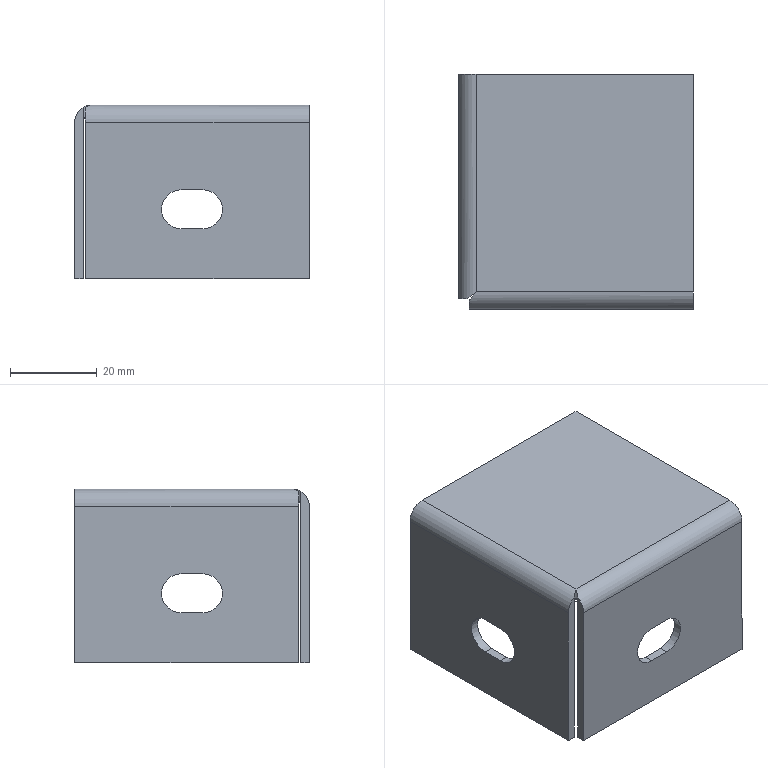Part | STEP file | 750038245 | 1 solid | 26 faces | box 54 x 54 x 40 mm | volume 12946 mm3 | plane 18 | cylinder 8 | commonest cylinder face diameters 9 x4 4 x2 8 x2
STEP:
#1=CARTESIAN_POINT('',(50.,50.,2.));
#2=VERTEX_POINT('',#1);
#3=CARTESIAN_POINT('',(50.,0.,2.));
#4=VERTEX_POINT('',#3);
#5=CARTESIAN_POINT('',(50.,0.,2.));
#6=DIRECTION('',(0.,-1.,0.));
#7=VECTOR('',#6,1000.);
#8=LINE('',#5,#7);
#9=EDGE_CURVE('',#2,#4,#8,.T.);
#10=ORIENTED_EDGE('',*,*,#9,.F.);
#11=CARTESIAN_POINT('',(0.,50.,2.));
#12=VERTEX_POINT('',#11);
#13=CARTESIAN_POINT('',(0.,50.,2.));
#14=DIRECTION('',(1.,0.,0.));
#15=VECTOR('',#14,1000.);
#16=LINE('',#13,#15);
#17=EDGE_CURVE('',#12,#2,#16,.T.);
#18=ORIENTED_EDGE('',*,*,#17,.F.);
#19=CARTESIAN_POINT('',(0.,0.,2.));
#20=VERTEX_POINT('',#19);
#21=CARTESIAN_POINT('',(0.,0.,2.));
#22=DIRECTION('',(0.,1.,0.));
#23=VECTOR('',#22,1000.);
#24=LINE('',#21,#23);
#25=EDGE_CURVE('',#20,#12,#24,.T.);
#26=ORIENTED_EDGE('',*,*,#25,.F.);
#27=CARTESIAN_POINT('',(0.,0.,2.));
#28=DIRECTION('',(-1.,0.,0.));
#29=VECTOR('',#28,1000.);
#30=LINE('',#27,#29);
#31=EDGE_CURVE('',#4,#20,#30,.T.);
#32=ORIENTED_EDGE('',*,*,#31,.F.);
#33=EDGE_LOOP('',(#10,#18,#26,#32));
#34=FACE_OUTER_BOUND('',#33,.T.);
#35=CARTESIAN_POINT('',(0.,0.,2.));
#36=DIRECTION('',(0.,0.,-1.));
#37=DIRECTION('',(-1.,0.,0.));
#38=AXIS2_PLACEMENT_3D('',#35,#36,#37);
#39=PLANE('',#38);
#40=ADVANCED_FACE('',(#34),#39,.F.);
#41=CARTESIAN_POINT('',(-1.5,-4.,-2.));
#42=VERTEX_POINT('',#41);
#43=CARTESIAN_POINT('',(50.,-4.,-2.));
#44=VERTEX_POINT('',#43);
#45=CARTESIAN_POINT('',(50.,-4.,-2.));
#46=DIRECTION('',(1.,0.,0.));
#47=VECTOR('',#46,1000.);
#48=LINE('',#45,#47);
#49=EDGE_CURVE('',#42,#44,#48,.T.);
#50=ORIENTED_EDGE('',*,*,#49,.T.);
#51=CARTESIAN_POINT('',(50.,0.,-2.));
#52=DIRECTION('',(-1.,0.,0.));
#53=DIRECTION('',(0.,0.,1.));
#54=AXIS2_PLACEMENT_3D('',#51,#52,#53);
#55=CIRCLE('',#54,4.);
#56=EDGE_CURVE('',#44,#4,#55,.T.);
#57=ORIENTED_EDGE('',*,*,#56,.T.);
#58=ORIENTED_EDGE('',*,*,#31,.T.);
#59=CARTESIAN_POINT('',(-1.5,-2.,1.464));
#60=VERTEX_POINT('',#59);
#61=CARTESIAN_POINT('',(0.,0.,2.));
#62=CARTESIAN_POINT('',(-0.5297,-0.7062,2.));
#63=CARTESIAN_POINT('',(-1.041,-1.388,1.817));
#64=CARTESIAN_POINT('',(-1.5,-2.,1.464));
#65=(BOUNDED_CURVE()B_SPLINE_CURVE(3,(#61,#62,#63,#64),.UNSPECIFIED.,.F.,.T.)B_SPLINE_CURVE_WITH_KNOTS((4,4),(4.712,5.236),.UNSPECIFIED.)CURVE()GEOMETRIC_REPRESENTATION_ITEM()RATIONAL_B_SPLINE_CURVE((1.,0.9773,0.9773,1.))REPRESENTATION_ITEM(''));
#66=EDGE_CURVE('',#20,#60,#65,.T.);
#67=ORIENTED_EDGE('',*,*,#66,.T.);
#68=CARTESIAN_POINT('',(-1.5,0.,-2.));
#69=DIRECTION('',(1.,0.,0.));
#70=DIRECTION('',(0.,0.,1.));
#71=AXIS2_PLACEMENT_3D('',#68,#69,#70);
#72=CIRCLE('',#71,4.);
#73=EDGE_CURVE('',#60,#42,#72,.T.);
#74=ORIENTED_EDGE('',*,*,#73,.T.);
#75=EDGE_LOOP('',(#50,#57,#58,#67,#74));
#76=FACE_OUTER_BOUND('',#75,.T.);
#77=CARTESIAN_POINT('',(50.,0.,-2.));
#78=DIRECTION('',(-1.,0.,0.));
#79=DIRECTION('',(0.,0.,1.));
#80=AXIS2_PLACEMENT_3D('',#77,#78,#79);
#81=CYLINDRICAL_SURFACE('',#80,4.);
#82=ADVANCED_FACE('',(#76),#81,.T.);
#83=CARTESIAN_POINT('',(50.,0.,0.));
#84=VERTEX_POINT('',#83);
#85=CARTESIAN_POINT('',(50.,50.,0.));
#86=VERTEX_POINT('',#85);
#87=CARTESIAN_POINT('',(50.,50.,0.));
#88=DIRECTION('',(0.,1.,0.));
#89=VECTOR('',#88,1000.);
#90=LINE('',#87,#89);
#91=EDGE_CURVE('',#84,#86,#90,.T.);
#92=ORIENTED_EDGE('',*,*,#91,.T.);
#93=CARTESIAN_POINT('',(50.,50.,2.));
#94=DIRECTION('',(0.,0.,1.));
#95=VECTOR('',#94,1000.);
#96=LINE('',#93,#95);
#97=EDGE_CURVE('',#86,#2,#96,.T.);
#98=ORIENTED_EDGE('',*,*,#97,.T.);
#99=ORIENTED_EDGE('',*,*,#9,.T.);
#100=ORIENTED_EDGE('',*,*,#56,.F.);
#101=CARTESIAN_POINT('',(50.,-4.,-38.));
#102=VERTEX_POINT('',#101);
#103=CARTESIAN_POINT('',(50.,-4.,2.));
#104=DIRECTION('',(0.,0.,-1.));
#105=VECTOR('',#104,1000.);
#106=LINE('',#103,#105);
#107=EDGE_CURVE('',#44,#102,#106,.T.);
#108=ORIENTED_EDGE('',*,*,#107,.T.);
#109=CARTESIAN_POINT('',(50.,-2.,-38.));
#110=VERTEX_POINT('',#109);
#111=CARTESIAN_POINT('',(50.,50.,-38.));
#112=DIRECTION('',(0.,1.,0.));
#113=VECTOR('',#112,1000.);
#114=LINE('',#111,#113);
#115=EDGE_CURVE('',#102,#110,#114,.T.);
#116=ORIENTED_EDGE('',*,*,#115,.T.);
#117=CARTESIAN_POINT('',(50.,-2.,-2.));
#118=VERTEX_POINT('',#117);
#119=CARTESIAN_POINT('',(50.,-2.,2.));
#120=DIRECTION('',(0.,0.,1.));
#121=VECTOR('',#120,1000.);
#122=LINE('',#119,#121);
#123=EDGE_CURVE('',#110,#118,#122,.T.);
#124=ORIENTED_EDGE('',*,*,#123,.T.);
#125=CARTESIAN_POINT('',(50.,0.,-2.));
#126=DIRECTION('',(-1.,0.,0.));
#127=DIRECTION('',(0.,0.,1.));
#128=AXIS2_PLACEMENT_3D('',#125,#126,#127);
#129=CIRCLE('',#128,2.);
#130=EDGE_CURVE('',#118,#84,#129,.T.);
#131=ORIENTED_EDGE('',*,*,#130,.T.);
#132=EDGE_LOOP('',(#92,#98,#99,#100,#108,#116,#124,#131));
#133=FACE_OUTER_BOUND('',#132,.T.);
#134=CARTESIAN_POINT('',(50.,50.,2.));
#135=DIRECTION('',(1.,0.,0.));
#136=DIRECTION('',(0.,1.,0.));
#137=AXIS2_PLACEMENT_3D('',#134,#135,#136);
#138=PLANE('',#137);
#139=ADVANCED_FACE('',(#133),#138,.T.);
#140=ORIENTED_EDGE('',*,*,#97,.F.);
#141=CARTESIAN_POINT('',(0.,50.,0.));
#142=VERTEX_POINT('',#141);
#143=CARTESIAN_POINT('',(0.,50.,0.));
#144=DIRECTION('',(-1.,0.,0.));
#145=VECTOR('',#144,1000.);
#146=LINE('',#143,#145);
#147=EDGE_CURVE('',#86,#142,#146,.T.);
#148=ORIENTED_EDGE('',*,*,#147,.T.);
#149=CARTESIAN_POINT('',(-2.,50.,-2.));
#150=VERTEX_POINT('',#149);
#151=CARTESIAN_POINT('',(0.,50.,-2.));
#152=DIRECTION('',(0.,-1.,0.));
#153=DIRECTION('',(-1.,0.,0.));
#154=AXIS2_PLACEMENT_3D('',#151,#152,#153);
#155=CIRCLE('',#154,2.);
#156=EDGE_CURVE('',#142,#150,#155,.T.);
#157=ORIENTED_EDGE('',*,*,#156,.T.);
#158=CARTESIAN_POINT('',(-2.,50.,-38.));
#159=VERTEX_POINT('',#158);
#160=CARTESIAN_POINT('',(-2.,50.,2.));
#161=DIRECTION('',(0.,0.,-1.));
#162=VECTOR('',#161,1000.);
#163=LINE('',#160,#162);
#164=EDGE_CURVE('',#150,#159,#163,.T.);
#165=ORIENTED_EDGE('',*,*,#164,.T.);
#166=CARTESIAN_POINT('',(-4.,50.,-38.));
#167=VERTEX_POINT('',#166);
#168=CARTESIAN_POINT('',(0.,50.,-38.));
#169=DIRECTION('',(-1.,0.,0.));
#170=VECTOR('',#169,1000.);
#171=LINE('',#168,#170);
#172=EDGE_CURVE('',#159,#167,#171,.T.);
#173=ORIENTED_EDGE('',*,*,#172,.T.);
#174=CARTESIAN_POINT('',(-4.,50.,-2.));
#175=VERTEX_POINT('',#174);
#176=CARTESIAN_POINT('',(-4.,50.,2.));
#177=DIRECTION('',(0.,0.,1.));
#178=VECTOR('',#177,1000.);
#179=LINE('',#176,#178);
#180=EDGE_CURVE('',#167,#175,#179,.T.);
#181=ORIENTED_EDGE('',*,*,#180,.T.);
#182=CARTESIAN_POINT('',(0.,50.,-2.));
#183=DIRECTION('',(0.,-1.,0.));
#184=DIRECTION('',(-1.,0.,0.));
#185=AXIS2_PLACEMENT_3D('',#182,#183,#184);
#186=CIRCLE('',#185,4.);
#187=EDGE_CURVE('',#12,#175,#186,.T.);
#188=ORIENTED_EDGE('',*,*,#187,.F.);
#189=ORIENTED_EDGE('',*,*,#17,.T.);
#190=EDGE_LOOP('',(#140,#148,#157,#165,#173,#181,#188,#189));
#191=FACE_OUTER_BOUND('',#190,.T.);
#192=CARTESIAN_POINT('',(0.,50.,2.));
#193=DIRECTION('',(0.,1.,0.));
#194=DIRECTION('',(0.,0.,1.));
#195=AXIS2_PLACEMENT_3D('',#192,#193,#194);
#196=PLANE('',#195);
#197=ADVANCED_FACE('',(#191),#196,.T.);
#198=CARTESIAN_POINT('',(-4.,-1.5,-2.));
#199=VERTEX_POINT('',#198);
#200=CARTESIAN_POINT('',(-4.,0.,-2.));
#201=DIRECTION('',(0.,-1.,0.));
#202=VECTOR('',#201,1000.);
#203=LINE('',#200,#202);
#204=EDGE_CURVE('',#175,#199,#203,.T.);
#205=ORIENTED_EDGE('',*,*,#204,.T.);
#206=CARTESIAN_POINT('',(-2.,-1.5,1.464));
#207=VERTEX_POINT('',#206);
#208=CARTESIAN_POINT('',(0.,-1.5,-2.));
#209=DIRECTION('',(0.,1.,0.));
#210=DIRECTION('',(-1.,0.,0.));
#211=AXIS2_PLACEMENT_3D('',#208,#209,#210);
#212=CIRCLE('',#211,4.);
#213=EDGE_CURVE('',#199,#207,#212,.T.);
#214=ORIENTED_EDGE('',*,*,#213,.T.);
#215=CARTESIAN_POINT('',(-2.,-1.5,1.464));
#216=CARTESIAN_POINT('',(-1.388,-1.041,1.817));
#217=CARTESIAN_POINT('',(-0.7062,-0.5297,2.));
#218=CARTESIAN_POINT('',(0.,0.,2.));
#219=(BOUNDED_CURVE()B_SPLINE_CURVE(3,(#215,#216,#217,#218),.UNSPECIFIED.,.F.,.F.)B_SPLINE_CURVE_WITH_KNOTS((4,4),(4.189,4.712),.UNSPECIFIED.)CURVE()GEOMETRIC_REPRESENTATION_ITEM()RATIONAL_B_SPLINE_CURVE((1.,0.9773,0.9773,1.))REPRESENTATION_ITEM(''));
#220=EDGE_CURVE('',#207,#20,#219,.T.);
#221=ORIENTED_EDGE('',*,*,#220,.T.);
#222=ORIENTED_EDGE('',*,*,#25,.T.);
#223=ORIENTED_EDGE('',*,*,#187,.T.);
#224=EDGE_LOOP('',(#205,#214,#221,#222,#223));
#225=FACE_OUTER_BOUND('',#224,.T.);
#226=CARTESIAN_POINT('',(0.,0.,-2.));
#227=DIRECTION('',(0.,1.,0.));
#228=DIRECTION('',(-1.,0.,0.));
#229=AXIS2_PLACEMENT_3D('',#226,#227,#228);
#230=CYLINDRICAL_SURFACE('',#229,4.);
#231=ADVANCED_FACE('',(#225),#230,.T.);
#232=CARTESIAN_POINT('',(-1.5,-4.,-38.));
#233=VERTEX_POINT('',#232);
#234=CARTESIAN_POINT('',(50.,-4.,-38.));
#235=DIRECTION('',(-1.,0.,0.));
#236=VECTOR('',#235,1000.);
#237=LINE('',#234,#236);
#238=EDGE_CURVE('',#102,#233,#237,.T.);
#239=ORIENTED_EDGE('',*,*,#238,.F.);
#240=ORIENTED_EDGE('',*,*,#107,.F.);
#241=ORIENTED_EDGE('',*,*,#49,.F.);
#242=CARTESIAN_POINT('',(-1.5,-4.,-2.));
#243=DIRECTION('',(0.,0.,1.));
#244=VECTOR('',#243,1000.);
#245=LINE('',#242,#244);
#246=EDGE_CURVE('',#233,#42,#245,.T.);
#247=ORIENTED_EDGE('',*,*,#246,.F.);
#248=EDGE_LOOP('',(#239,#240,#241,#247));
#249=FACE_OUTER_BOUND('',#248,.T.);
#250=CARTESIAN_POINT('',(25.5,-4.,-17.5));
#251=VERTEX_POINT('',#250);
#252=CARTESIAN_POINT('',(20.5,-4.,-17.5));
#253=VERTEX_POINT('',#252);
#254=CARTESIAN_POINT('',(50.,-4.,-17.5));
#255=DIRECTION('',(-1.,0.,0.));
#256=VECTOR('',#255,1000.);
#257=LINE('',#254,#256);
#258=EDGE_CURVE('',#251,#253,#257,.T.);
#259=ORIENTED_EDGE('',*,*,#258,.F.);
#260=CARTESIAN_POINT('',(25.5,-4.,-26.5));
#261=VERTEX_POINT('',#260);
#262=CARTESIAN_POINT('',(25.5,-4.,-22.));
#263=DIRECTION('',(0.,-1.,0.));
#264=DIRECTION('',(0.,0.,-1.));
#265=AXIS2_PLACEMENT_3D('',#262,#263,#264);
#266=CIRCLE('',#265,4.5);
#267=EDGE_CURVE('',#261,#251,#266,.T.);
#268=ORIENTED_EDGE('',*,*,#267,.F.);
#269=CARTESIAN_POINT('',(20.5,-4.,-26.5));
#270=VERTEX_POINT('',#269);
#271=CARTESIAN_POINT('',(50.,-4.,-26.5));
#272=DIRECTION('',(1.,0.,0.));
#273=VECTOR('',#272,1000.);
#274=LINE('',#271,#273);
#275=EDGE_CURVE('',#270,#261,#274,.T.);
#276=ORIENTED_EDGE('',*,*,#275,.F.);
#277=CARTESIAN_POINT('',(20.5,-4.,-22.));
#278=DIRECTION('',(0.,-1.,0.));
#279=DIRECTION('',(0.,0.,-1.));
#280=AXIS2_PLACEMENT_3D('',#277,#278,#279);
#281=CIRCLE('',#280,4.5);
#282=EDGE_CURVE('',#253,#270,#281,.T.);
#283=ORIENTED_EDGE('',*,*,#282,.F.);
#284=EDGE_LOOP('',(#259,#268,#276,#283));
#285=FACE_BOUND('',#284,.T.);
#286=CARTESIAN_POINT('',(50.,-4.,-2.));
#287=DIRECTION('',(0.,1.,0.));
#288=DIRECTION('',(0.,0.,1.));
#289=AXIS2_PLACEMENT_3D('',#286,#287,#288);
#290=PLANE('',#289);
#291=ADVANCED_FACE('',(#249,#285),#290,.F.);
#292=CARTESIAN_POINT('',(-1.5,-2.,-2.));
#293=VERTEX_POINT('',#292);
#294=CARTESIAN_POINT('',(-1.5,-2.,-38.));
#295=VERTEX_POINT('',#294);
#296=CARTESIAN_POINT('',(-1.5,-2.,2.));
#297=DIRECTION('',(0.,0.,-1.));
#298=VECTOR('',#297,1000.);
#299=LINE('',#296,#298);
#300=EDGE_CURVE('',#293,#295,#299,.T.);
#301=ORIENTED_EDGE('',*,*,#300,.T.);
#302=CARTESIAN_POINT('',(-1.5,0.,-38.));
#303=DIRECTION('',(0.,-1.,0.));
#304=VECTOR('',#303,1000.);
#305=LINE('',#302,#304);
#306=EDGE_CURVE('',#295,#233,#305,.T.);
#307=ORIENTED_EDGE('',*,*,#306,.T.);
#308=ORIENTED_EDGE('',*,*,#246,.T.);
#309=ORIENTED_EDGE('',*,*,#73,.F.);
#310=CARTESIAN_POINT('',(-1.5,-2.,2.));
#311=DIRECTION('',(0.,0.,-1.));
#312=VECTOR('',#311,1000.);
#313=LINE('',#310,#312);
#314=EDGE_CURVE('',#60,#293,#313,.T.);
#315=ORIENTED_EDGE('',*,*,#314,.T.);
#316=EDGE_LOOP('',(#301,#307,#308,#309,#315));
#317=FACE_OUTER_BOUND('',#316,.T.);
#318=CARTESIAN_POINT('',(-1.5,0.,2.));
#319=DIRECTION('',(-1.,0.,0.));
#320=DIRECTION('',(0.,-1.,0.));
#321=AXIS2_PLACEMENT_3D('',#318,#319,#320);
#322=PLANE('',#321);
#323=ADVANCED_FACE('',(#317),#322,.T.);
#324=CARTESIAN_POINT('',(0.,0.,0.));
#325=VERTEX_POINT('',#324);
#326=CARTESIAN_POINT('',(-1.5,-2.,-2.));
#327=CARTESIAN_POINT('',(-1.5,-2.,-0.8284));
#328=CARTESIAN_POINT('',(-0.8787,-1.172,0.));
#329=CARTESIAN_POINT('',(0.,0.,0.));
#330=(BOUNDED_CURVE()B_SPLINE_CURVE(3,(#326,#327,#328,#329),.UNSPECIFIED.,.F.,.F.)B_SPLINE_CURVE_WITH_KNOTS((4,4),(0.,1.571),.UNSPECIFIED.)CURVE()GEOMETRIC_REPRESENTATION_ITEM()RATIONAL_B_SPLINE_CURVE((1.,0.8047,0.8047,1.))REPRESENTATION_ITEM(''));
#331=EDGE_CURVE('',#293,#325,#330,.T.);
#332=ORIENTED_EDGE('',*,*,#331,.F.);
#333=ORIENTED_EDGE('',*,*,#314,.F.);
#334=ORIENTED_EDGE('',*,*,#66,.F.);
#335=CARTESIAN_POINT('',(0.,0.,1002.));
#336=DIRECTION('',(0.,0.,1.));
#337=VECTOR('',#336,1000.);
#338=LINE('',#335,#337);
#339=EDGE_CURVE('',#325,#20,#338,.T.);
#340=ORIENTED_EDGE('',*,*,#339,.F.);
#341=EDGE_LOOP('',(#332,#333,#334,#340));
#342=FACE_OUTER_BOUND('',#341,.T.);
#343=CARTESIAN_POINT('',(600.,800.,1002.));
#344=DIRECTION('',(0.8,-0.6,0.));
#345=DIRECTION('',(0.6,0.8,0.));
#346=AXIS2_PLACEMENT_3D('',#343,#344,#345);
#347=PLANE('',#346);
#348=ADVANCED_FACE('',(#342),#347,.F.);
#349=ORIENTED_EDGE('',*,*,#147,.F.);
#350=ORIENTED_EDGE('',*,*,#91,.F.);
#351=CARTESIAN_POINT('',(0.,0.,0.));
#352=DIRECTION('',(-1.,0.,0.));
#353=VECTOR('',#352,1000.);
#354=LINE('',#351,#353);
#355=EDGE_CURVE('',#84,#325,#354,.T.);
#356=ORIENTED_EDGE('',*,*,#355,.T.);
#357=CARTESIAN_POINT('',(0.,0.,0.));
#358=DIRECTION('',(0.,1.,0.));
#359=VECTOR('',#358,1000.);
#360=LINE('',#357,#359);
#361=EDGE_CURVE('',#325,#142,#360,.T.);
#362=ORIENTED_EDGE('',*,*,#361,.T.);
#363=EDGE_LOOP('',(#349,#350,#356,#362));
#364=FACE_OUTER_BOUND('',#363,.T.);
#365=CARTESIAN_POINT('',(0.,0.,0.));
#366=DIRECTION('',(0.,0.,-1.));
#367=DIRECTION('',(-1.,0.,0.));
#368=AXIS2_PLACEMENT_3D('',#365,#366,#367);
#369=PLANE('',#368);
#370=ADVANCED_FACE('',(#364),#369,.T.);
#371=CARTESIAN_POINT('',(-4.,-1.5,-38.));
#372=VERTEX_POINT('',#371);
#373=CARTESIAN_POINT('',(-4.,-1.5,-2.));
#374=DIRECTION('',(0.,0.,-1.));
#375=VECTOR('',#374,1000.);
#376=LINE('',#373,#375);
#377=EDGE_CURVE('',#199,#372,#376,.T.);
#378=ORIENTED_EDGE('',*,*,#377,.T.);
#379=CARTESIAN_POINT('',(-2.,-1.5,-38.));
#380=VERTEX_POINT('',#379);
#381=CARTESIAN_POINT('',(-2.,-1.5,-38.));
#382=DIRECTION('',(1.,0.,0.));
#383=VECTOR('',#382,1000.);
#384=LINE('',#381,#383);
#385=EDGE_CURVE('',#372,#380,#384,.T.);
#386=ORIENTED_EDGE('',*,*,#385,.T.);
#387=CARTESIAN_POINT('',(-2.,-1.5,-2.));
#388=VERTEX_POINT('',#387);
#389=CARTESIAN_POINT('',(-2.,-1.5,-2.));
#390=DIRECTION('',(0.,0.,1.));
#391=VECTOR('',#390,1000.);
#392=LINE('',#389,#391);
#393=EDGE_CURVE('',#380,#388,#392,.T.);
#394=ORIENTED_EDGE('',*,*,#393,.T.);
#395=CARTESIAN_POINT('',(-2.,-1.5,-2.));
#396=DIRECTION('',(0.,0.,1.));
#397=VECTOR('',#396,1000.);
#398=LINE('',#395,#397);
#399=EDGE_CURVE('',#388,#207,#398,.T.);
#400=ORIENTED_EDGE('',*,*,#399,.T.);
#401=ORIENTED_EDGE('',*,*,#213,.F.);
#402=EDGE_LOOP('',(#378,#386,#394,#400,#401));
#403=FACE_OUTER_BOUND('',#402,.T.);
#404=CARTESIAN_POINT('',(-2.,-1.5,-2.));
#405=DIRECTION('',(0.,-1.,0.));
#406=DIRECTION('',(1.,0.,0.));
#407=AXIS2_PLACEMENT_3D('',#404,#405,#406);
#408=PLANE('',#407);
#409=ADVANCED_FACE('',(#403),#408,.T.);
#410=CARTESIAN_POINT('',(-4.,0.,-38.));
#411=DIRECTION('',(0.,1.,0.));
#412=VECTOR('',#411,1000.);
#413=LINE('',#410,#412);
#414=EDGE_CURVE('',#372,#167,#413,.T.);
#415=ORIENTED_EDGE('',*,*,#414,.F.);
#416=ORIENTED_EDGE('',*,*,#377,.F.);
#417=ORIENTED_EDGE('',*,*,#204,.F.);
#418=ORIENTED_EDGE('',*,*,#180,.F.);
#419=EDGE_LOOP('',(#415,#416,#417,#418));
#420=FACE_OUTER_BOUND('',#419,.T.);
#421=CARTESIAN_POINT('',(-4.,25.5,-26.5));
#422=VERTEX_POINT('',#421);
#423=CARTESIAN_POINT('',(-4.,20.5,-26.5));
#424=VERTEX_POINT('',#423);
#425=CARTESIAN_POINT('',(-4.,0.,-26.5));
#426=DIRECTION('',(0.,-1.,0.));
#427=VECTOR('',#426,1000.);
#428=LINE('',#425,#427);
#429=EDGE_CURVE('',#422,#424,#428,.T.);
#430=ORIENTED_EDGE('',*,*,#429,.F.);
#431=CARTESIAN_POINT('',(-4.,25.5,-17.5));
#432=VERTEX_POINT('',#431);
#433=CARTESIAN_POINT('',(-4.,25.5,-22.));
#434=DIRECTION('',(-1.,0.,0.));
#435=DIRECTION('',(0.,0.,1.));
#436=AXIS2_PLACEMENT_3D('',#433,#434,#435);
#437=CIRCLE('',#436,4.5);
#438=EDGE_CURVE('',#432,#422,#437,.T.);
#439=ORIENTED_EDGE('',*,*,#438,.F.);
#440=CARTESIAN_POINT('',(-4.,20.5,-17.5));
#441=VERTEX_POINT('',#440);
#442=CARTESIAN_POINT('',(-4.,0.,-17.5));
#443=DIRECTION('',(0.,1.,0.));
#444=VECTOR('',#443,1000.);
#445=LINE('',#442,#444);
#446=EDGE_CURVE('',#441,#432,#445,.T.);
#447=ORIENTED_EDGE('',*,*,#446,.F.);
#448=CARTESIAN_POINT('',(-4.,20.5,-22.));
#449=DIRECTION('',(-1.,0.,0.));
#450=DIRECTION('',(0.,0.,1.));
#451=AXIS2_PLACEMENT_3D('',#448,#449,#450);
#452=CIRCLE('',#451,4.5);
#453=EDGE_CURVE('',#424,#441,#452,.T.);
#454=ORIENTED_EDGE('',*,*,#453,.F.);
#455=EDGE_LOOP('',(#430,#439,#447,#454));
#456=FACE_BOUND('',#455,.T.);
#457=CARTESIAN_POINT('',(-4.,0.,-2.));
#458=DIRECTION('',(1.,0.,0.));
#459=DIRECTION('',(0.,0.,-1.));
#460=AXIS2_PLACEMENT_3D('',#457,#458,#459);
#461=PLANE('',#460);
#462=ADVANCED_FACE('',(#420,#456),#461,.F.);
#463=ORIENTED_EDGE('',*,*,#220,.F.);
#464=ORIENTED_EDGE('',*,*,#399,.F.);
#465=CARTESIAN_POINT('',(-2.,-1.5,-2.));
#466=CARTESIAN_POINT('',(-2.,-1.5,-0.8284));
#467=CARTESIAN_POINT('',(-1.172,-0.8787,0.));
#468=CARTESIAN_POINT('',(0.,0.,0.));
#469=(BOUNDED_CURVE()B_SPLINE_CURVE(3,(#465,#466,#467,#468),.UNSPECIFIED.,.F.,.F.)B_SPLINE_CURVE_WITH_KNOTS((4,4),(3.142,4.712),.UNSPECIFIED.)CURVE()GEOMETRIC_REPRESENTATION_ITEM()RATIONAL_B_SPLINE_CURVE((1.,0.8047,0.8047,1.))REPRESENTATION_ITEM(''));
#470=EDGE_CURVE('',#388,#325,#469,.T.);
#471=ORIENTED_EDGE('',*,*,#470,.T.);
#472=ORIENTED_EDGE('',*,*,#339,.T.);
#473=EDGE_LOOP('',(#463,#464,#471,#472));
#474=FACE_OUTER_BOUND('',#473,.T.);
#475=CARTESIAN_POINT('',(800.,600.,1002.));
#476=DIRECTION('',(0.6,-0.8,0.));
#477=DIRECTION('',(0.8,0.6,0.));
#478=AXIS2_PLACEMENT_3D('',#475,#476,#477);
#479=PLANE('',#478);
#480=ADVANCED_FACE('',(#474),#479,.T.);
#481=ORIENTED_EDGE('',*,*,#306,.F.);
#482=CARTESIAN_POINT('',(50.,-2.,-38.));
#483=DIRECTION('',(1.,0.,0.));
#484=VECTOR('',#483,1000.);
#485=LINE('',#482,#484);
#486=EDGE_CURVE('',#295,#110,#485,.T.);
#487=ORIENTED_EDGE('',*,*,#486,.T.);
#488=ORIENTED_EDGE('',*,*,#115,.F.);
#489=ORIENTED_EDGE('',*,*,#238,.T.);
#490=EDGE_LOOP('',(#481,#487,#488,#489));
#491=FACE_OUTER_BOUND('',#490,.T.);
#492=CARTESIAN_POINT('',(50.,-2.,-38.));
#493=DIRECTION('',(0.,0.,-1.));
#494=DIRECTION('',(0.,1.,0.));
#495=AXIS2_PLACEMENT_3D('',#492,#493,#494);
#496=PLANE('',#495);
#497=ADVANCED_FACE('',(#491),#496,.T.);
#498=ORIENTED_EDGE('',*,*,#355,.F.);
#499=ORIENTED_EDGE('',*,*,#130,.F.);
#500=CARTESIAN_POINT('',(50.,-2.,-2.));
#501=DIRECTION('',(1.,0.,0.));
#502=VECTOR('',#501,1000.);
#503=LINE('',#500,#502);
#504=EDGE_CURVE('',#293,#118,#503,.T.);
#505=ORIENTED_EDGE('',*,*,#504,.F.);
#506=ORIENTED_EDGE('',*,*,#331,.T.);
#507=EDGE_LOOP('',(#498,#499,#505,#506));
#508=FACE_OUTER_BOUND('',#507,.T.);
#509=CARTESIAN_POINT('',(50.,0.,-2.));
#510=DIRECTION('',(-1.,0.,0.));
#511=DIRECTION('',(0.,0.,1.));
#512=AXIS2_PLACEMENT_3D('',#509,#510,#511);
#513=CYLINDRICAL_SURFACE('',#512,2.);
#514=ADVANCED_FACE('',(#508),#513,.F.);
#515=ORIENTED_EDGE('',*,*,#123,.F.);
#516=ORIENTED_EDGE('',*,*,#486,.F.);
#517=ORIENTED_EDGE('',*,*,#300,.F.);
#518=ORIENTED_EDGE('',*,*,#504,.T.);
#519=EDGE_LOOP('',(#515,#516,#517,#518));
#520=FACE_OUTER_BOUND('',#519,.T.);
#521=CARTESIAN_POINT('',(20.5,-2.,-26.5));
#522=VERTEX_POINT('',#521);
#523=CARTESIAN_POINT('',(25.5,-2.,-26.5));
#524=VERTEX_POINT('',#523);
#525=CARTESIAN_POINT('',(50.,-2.,-26.5));
#526=DIRECTION('',(1.,0.,0.));
#527=VECTOR('',#526,1000.);
#528=LINE('',#525,#527);
#529=EDGE_CURVE('',#522,#524,#528,.T.);
#530=ORIENTED_EDGE('',*,*,#529,.T.);
#531=CARTESIAN_POINT('',(25.5,-2.,-17.5));
#532=VERTEX_POINT('',#531);
#533=CARTESIAN_POINT('',(25.5,-2.,-22.));
#534=DIRECTION('',(0.,-1.,0.));
#535=DIRECTION('',(0.,0.,-1.));
#536=AXIS2_PLACEMENT_3D('',#533,#534,#535);
#537=CIRCLE('',#536,4.5);
#538=EDGE_CURVE('',#524,#532,#537,.T.);
#539=ORIENTED_EDGE('',*,*,#538,.T.);
#540=CARTESIAN_POINT('',(20.5,-2.,-17.5));
#541=VERTEX_POINT('',#540);
#542=CARTESIAN_POINT('',(50.,-2.,-17.5));
#543=DIRECTION('',(-1.,0.,0.));
#544=VECTOR('',#543,1000.);
#545=LINE('',#542,#544);
#546=EDGE_CURVE('',#532,#541,#545,.T.);
#547=ORIENTED_EDGE('',*,*,#546,.T.);
#548=CARTESIAN_POINT('',(20.5,-2.,-22.));
#549=DIRECTION('',(0.,-1.,0.));
#550=DIRECTION('',(0.,0.,-1.));
#551=AXIS2_PLACEMENT_3D('',#548,#549,#550);
#552=CIRCLE('',#551,4.5);
#553=EDGE_CURVE('',#541,#522,#552,.T.);
#554=ORIENTED_EDGE('',*,*,#553,.T.);
#555=EDGE_LOOP('',(#530,#539,#547,#554));
#556=FACE_BOUND('',#555,.T.);
#557=CARTESIAN_POINT('',(50.,-2.,-2.));
#558=DIRECTION('',(0.,1.,0.));
#559=DIRECTION('',(0.,0.,1.));
#560=AXIS2_PLACEMENT_3D('',#557,#558,#559);
#561=PLANE('',#560);
#562=ADVANCED_FACE('',(#520,#556),#561,.T.);
#563=CARTESIAN_POINT('',(20.5,82.209,-17.5));
#564=DIRECTION('',(0.,1.,0.));
#565=VECTOR('',#564,1000.);
#566=LINE('',#563,#565);
#567=EDGE_CURVE('',#253,#541,#566,.T.);
#568=ORIENTED_EDGE('',*,*,#567,.F.);
#569=ORIENTED_EDGE('',*,*,#282,.T.);
#570=CARTESIAN_POINT('',(20.5,82.209,-26.5));
#571=DIRECTION('',(0.,-1.,0.));
#572=VECTOR('',#571,1000.);
#573=LINE('',#570,#572);
#574=EDGE_CURVE('',#522,#270,#573,.T.);
#575=ORIENTED_EDGE('',*,*,#574,.F.);
#576=ORIENTED_EDGE('',*,*,#553,.F.);
#577=EDGE_LOOP('',(#568,#569,#575,#576));
#578=FACE_OUTER_BOUND('',#577,.T.);
#579=CARTESIAN_POINT('',(20.5,82.209,-22.));
#580=DIRECTION('',(0.,-1.,0.));
#581=DIRECTION('',(0.,0.,-1.));
#582=AXIS2_PLACEMENT_3D('',#579,#580,#581);
#583=CYLINDRICAL_SURFACE('',#582,4.5);
#584=ADVANCED_FACE('',(#578),#583,.F.);
#585=CARTESIAN_POINT('',(25.5,82.209,-17.5));
#586=DIRECTION('',(0.,1.,0.));
#587=VECTOR('',#586,1000.);
#588=LINE('',#585,#587);
#589=EDGE_CURVE('',#251,#532,#588,.T.);
#590=ORIENTED_EDGE('',*,*,#589,.F.);
#591=ORIENTED_EDGE('',*,*,#258,.T.);
#592=ORIENTED_EDGE('',*,*,#567,.T.);
#593=ORIENTED_EDGE('',*,*,#546,.F.);
#594=EDGE_LOOP('',(#590,#591,#592,#593));
#595=FACE_OUTER_BOUND('',#594,.T.);
#596=CARTESIAN_POINT('',(25.5,82.209,-17.5));
#597=DIRECTION('',(0.,0.,1.));
#598=DIRECTION('',(1.,0.,0.));
#599=AXIS2_PLACEMENT_3D('',#596,#597,#598);
#600=PLANE('',#599);
#601=ADVANCED_FACE('',(#595),#600,.F.);
#602=CARTESIAN_POINT('',(25.5,82.209,-26.5));
#603=DIRECTION('',(0.,1.,0.));
#604=VECTOR('',#603,1000.);
#605=LINE('',#602,#604);
#606=EDGE_CURVE('',#261,#524,#605,.T.);
#607=ORIENTED_EDGE('',*,*,#606,.F.);
#608=ORIENTED_EDGE('',*,*,#267,.T.);
#609=ORIENTED_EDGE('',*,*,#589,.T.);
#610=ORIENTED_EDGE('',*,*,#538,.F.);
#611=EDGE_LOOP('',(#607,#608,#609,#610));
#612=FACE_OUTER_BOUND('',#611,.T.);
#613=CARTESIAN_POINT('',(25.5,82.209,-22.));
#614=DIRECTION('',(0.,-1.,0.));
#615=DIRECTION('',(0.,0.,-1.));
#616=AXIS2_PLACEMENT_3D('',#613,#614,#615);
#617=CYLINDRICAL_SURFACE('',#616,4.5);
#618=ADVANCED_FACE('',(#612),#617,.F.);
#619=ORIENTED_EDGE('',*,*,#574,.T.);
#620=ORIENTED_EDGE('',*,*,#275,.T.);
#621=ORIENTED_EDGE('',*,*,#606,.T.);
#622=ORIENTED_EDGE('',*,*,#529,.F.);
#623=EDGE_LOOP('',(#619,#620,#621,#622));
#624=FACE_OUTER_BOUND('',#623,.T.);
#625=CARTESIAN_POINT('',(20.5,82.209,-26.5));
#626=DIRECTION('',(0.,0.,-1.));
#627=DIRECTION('',(-1.,0.,0.));
#628=AXIS2_PLACEMENT_3D('',#625,#626,#627);
#629=PLANE('',#628);
#630=ADVANCED_FACE('',(#624),#629,.F.);
#631=ORIENTED_EDGE('',*,*,#470,.F.);
#632=CARTESIAN_POINT('',(-2.,0.,-2.));
#633=DIRECTION('',(0.,-1.,0.));
#634=VECTOR('',#633,1000.);
#635=LINE('',#632,#634);
#636=EDGE_CURVE('',#150,#388,#635,.T.);
#637=ORIENTED_EDGE('',*,*,#636,.F.);
#638=ORIENTED_EDGE('',*,*,#156,.F.);
#639=ORIENTED_EDGE('',*,*,#361,.F.);
#640=EDGE_LOOP('',(#631,#637,#638,#639));
#641=FACE_OUTER_BOUND('',#640,.T.);
#642=CARTESIAN_POINT('',(0.,0.,-2.));
#643=DIRECTION('',(0.,1.,0.));
#644=DIRECTION('',(-1.,0.,0.));
#645=AXIS2_PLACEMENT_3D('',#642,#643,#644);
#646=CYLINDRICAL_SURFACE('',#645,2.);
#647=ADVANCED_FACE('',(#641),#646,.F.);
#648=ORIENTED_EDGE('',*,*,#172,.F.);
#649=CARTESIAN_POINT('',(-2.,0.,-38.));
#650=DIRECTION('',(0.,-1.,0.));
#651=VECTOR('',#650,1000.);
#652=LINE('',#649,#651);
#653=EDGE_CURVE('',#159,#380,#652,.T.);
#654=ORIENTED_EDGE('',*,*,#653,.T.);
#655=ORIENTED_EDGE('',*,*,#385,.F.);
#656=ORIENTED_EDGE('',*,*,#414,.T.);
#657=EDGE_LOOP('',(#648,#654,#655,#656));
#658=FACE_OUTER_BOUND('',#657,.T.);
#659=CARTESIAN_POINT('',(-2.,0.,-38.));
#660=DIRECTION('',(0.,0.,-1.));
#661=DIRECTION('',(-1.,0.,0.));
#662=AXIS2_PLACEMENT_3D('',#659,#660,#661);
#663=PLANE('',#662);
#664=ADVANCED_FACE('',(#658),#663,.T.);
#665=ORIENTED_EDGE('',*,*,#393,.F.);
#666=ORIENTED_EDGE('',*,*,#653,.F.);
#667=ORIENTED_EDGE('',*,*,#164,.F.);
#668=ORIENTED_EDGE('',*,*,#636,.T.);
#669=EDGE_LOOP('',(#665,#666,#667,#668));
#670=FACE_OUTER_BOUND('',#669,.T.);
#671=CARTESIAN_POINT('',(-2.,20.5,-17.5));
#672=VERTEX_POINT('',#671);
#673=CARTESIAN_POINT('',(-2.,25.5,-17.5));
#674=VERTEX_POINT('',#673);
#675=CARTESIAN_POINT('',(-2.,0.,-17.5));
#676=DIRECTION('',(0.,1.,0.));
#677=VECTOR('',#676,1000.);
#678=LINE('',#675,#677);
#679=EDGE_CURVE('',#672,#674,#678,.T.);
#680=ORIENTED_EDGE('',*,*,#679,.T.);
#681=CARTESIAN_POINT('',(-2.,25.5,-26.5));
#682=VERTEX_POINT('',#681);
#683=CARTESIAN_POINT('',(-2.,25.5,-22.));
#684=DIRECTION('',(-1.,0.,0.));
#685=DIRECTION('',(0.,0.,1.));
#686=AXIS2_PLACEMENT_3D('',#683,#684,#685);
#687=CIRCLE('',#686,4.5);
#688=EDGE_CURVE('',#674,#682,#687,.T.);
#689=ORIENTED_EDGE('',*,*,#688,.T.);
#690=CARTESIAN_POINT('',(-2.,20.5,-26.5));
#691=VERTEX_POINT('',#690);
#692=CARTESIAN_POINT('',(-2.,0.,-26.5));
#693=DIRECTION('',(0.,-1.,0.));
#694=VECTOR('',#693,1000.);
#695=LINE('',#692,#694);
#696=EDGE_CURVE('',#682,#691,#695,.T.);
#697=ORIENTED_EDGE('',*,*,#696,.T.);
#698=CARTESIAN_POINT('',(-2.,20.5,-22.));
#699=DIRECTION('',(-1.,0.,0.));
#700=DIRECTION('',(0.,0.,1.));
#701=AXIS2_PLACEMENT_3D('',#698,#699,#700);
#702=CIRCLE('',#701,4.5);
#703=EDGE_CURVE('',#691,#672,#702,.T.);
#704=ORIENTED_EDGE('',*,*,#703,.T.);
#705=EDGE_LOOP('',(#680,#689,#697,#704));
#706=FACE_BOUND('',#705,.T.);
#707=CARTESIAN_POINT('',(-2.,0.,-2.));
#708=DIRECTION('',(1.,0.,0.));
#709=DIRECTION('',(0.,0.,-1.));
#710=AXIS2_PLACEMENT_3D('',#707,#708,#709);
#711=PLANE('',#710);
#712=ADVANCED_FACE('',(#670,#706),#711,.T.);
#713=CARTESIAN_POINT('',(82.209,20.5,-26.5));
#714=DIRECTION('',(1.,0.,0.));
#715=VECTOR('',#714,1000.);
#716=LINE('',#713,#715);
#717=EDGE_CURVE('',#424,#691,#716,.T.);
#718=ORIENTED_EDGE('',*,*,#717,.F.);
#719=ORIENTED_EDGE('',*,*,#453,.T.);
#720=CARTESIAN_POINT('',(82.209,20.5,-17.5));
#721=DIRECTION('',(-1.,0.,0.));
#722=VECTOR('',#721,1000.);
#723=LINE('',#720,#722);
#724=EDGE_CURVE('',#672,#441,#723,.T.);
#725=ORIENTED_EDGE('',*,*,#724,.F.);
#726=ORIENTED_EDGE('',*,*,#703,.F.);
#727=EDGE_LOOP('',(#718,#719,#725,#726));
#728=FACE_OUTER_BOUND('',#727,.T.);
#729=CARTESIAN_POINT('',(82.209,20.5,-22.));
#730=DIRECTION('',(-1.,0.,0.));
#731=DIRECTION('',(0.,0.,1.));
#732=AXIS2_PLACEMENT_3D('',#729,#730,#731);
#733=CYLINDRICAL_SURFACE('',#732,4.5);
#734=ADVANCED_FACE('',(#728),#733,.F.);
#735=CARTESIAN_POINT('',(82.209,25.5,-26.5));
#736=DIRECTION('',(1.,0.,0.));
#737=VECTOR('',#736,1000.);
#738=LINE('',#735,#737);
#739=EDGE_CURVE('',#422,#682,#738,.T.);
#740=ORIENTED_EDGE('',*,*,#739,.F.);
#741=ORIENTED_EDGE('',*,*,#429,.T.);
#742=ORIENTED_EDGE('',*,*,#717,.T.);
#743=ORIENTED_EDGE('',*,*,#696,.F.);
#744=EDGE_LOOP('',(#740,#741,#742,#743));
#745=FACE_OUTER_BOUND('',#744,.T.);
#746=CARTESIAN_POINT('',(82.209,25.5,-26.5));
#747=DIRECTION('',(0.,0.,-1.));
#748=DIRECTION('',(-1.,0.,0.));
#749=AXIS2_PLACEMENT_3D('',#746,#747,#748);
#750=PLANE('',#749);
#751=ADVANCED_FACE('',(#745),#750,.F.);
#752=CARTESIAN_POINT('',(82.209,25.5,-17.5));
#753=DIRECTION('',(1.,0.,0.));
#754=VECTOR('',#753,1000.);
#755=LINE('',#752,#754);
#756=EDGE_CURVE('',#432,#674,#755,.T.);
#757=ORIENTED_EDGE('',*,*,#756,.F.);
#758=ORIENTED_EDGE('',*,*,#438,.T.);
#759=ORIENTED_EDGE('',*,*,#739,.T.);
#760=ORIENTED_EDGE('',*,*,#688,.F.);
#761=EDGE_LOOP('',(#757,#758,#759,#760));
#762=FACE_OUTER_BOUND('',#761,.T.);
#763=CARTESIAN_POINT('',(82.209,25.5,-22.));
#764=DIRECTION('',(-1.,0.,0.));
#765=DIRECTION('',(0.,0.,1.));
#766=AXIS2_PLACEMENT_3D('',#763,#764,#765);
#767=CYLINDRICAL_SURFACE('',#766,4.5);
#768=ADVANCED_FACE('',(#762),#767,.F.);
#769=ORIENTED_EDGE('',*,*,#724,.T.);
#770=ORIENTED_EDGE('',*,*,#446,.T.);
#771=ORIENTED_EDGE('',*,*,#756,.T.);
#772=ORIENTED_EDGE('',*,*,#679,.F.);
#773=EDGE_LOOP('',(#769,#770,#771,#772));
#774=FACE_OUTER_BOUND('',#773,.T.);
#775=CARTESIAN_POINT('',(82.209,20.5,-17.5));
#776=DIRECTION('',(0.,0.,1.));
#777=DIRECTION('',(1.,0.,0.));
#778=AXIS2_PLACEMENT_3D('',#775,#776,#777);
#779=PLANE('',#778);
#780=ADVANCED_FACE('',(#774),#779,.F.);
#781=CLOSED_SHELL('',(#40,#82,#139,#197,#231,#291,#323,#348,#370,#409,#462,#480,#497,#514,#562,#584,#601,#618,#630,#647,#664,#712,#734,#751,#768,#780));
#782=MANIFOLD_SOLID_BREP('',#781);
#783=CARTESIAN_POINT('',(0.,0.,0.));
#784=DIRECTION('',(0.,0.,1.));
#785=DIRECTION('',(1.,0.,0.));
#786=AXIS2_PLACEMENT_3D('',#783,#784,#785);
#787=(LENGTH_UNIT()NAMED_UNIT(*)SI_UNIT(.MILLI.,.METRE.));
#788=UNCERTAINTY_MEASURE_WITH_UNIT(LENGTH_MEASURE(0.00001),#787,'','');
#789=(NAMED_UNIT(*)PLANE_ANGLE_UNIT()SI_UNIT($,.RADIAN.));
#790=(NAMED_UNIT(*)SI_UNIT($,.STERADIAN.)SOLID_ANGLE_UNIT());
#791=(GEOMETRIC_REPRESENTATION_CONTEXT(3)GLOBAL_UNCERTAINTY_ASSIGNED_CONTEXT((#788))GLOBAL_UNIT_ASSIGNED_CONTEXT((#787,#789,#790))REPRESENTATION_CONTEXT('',''));
#792=ADVANCED_BREP_SHAPE_REPRESENTATION('',(#782,#786),#791);